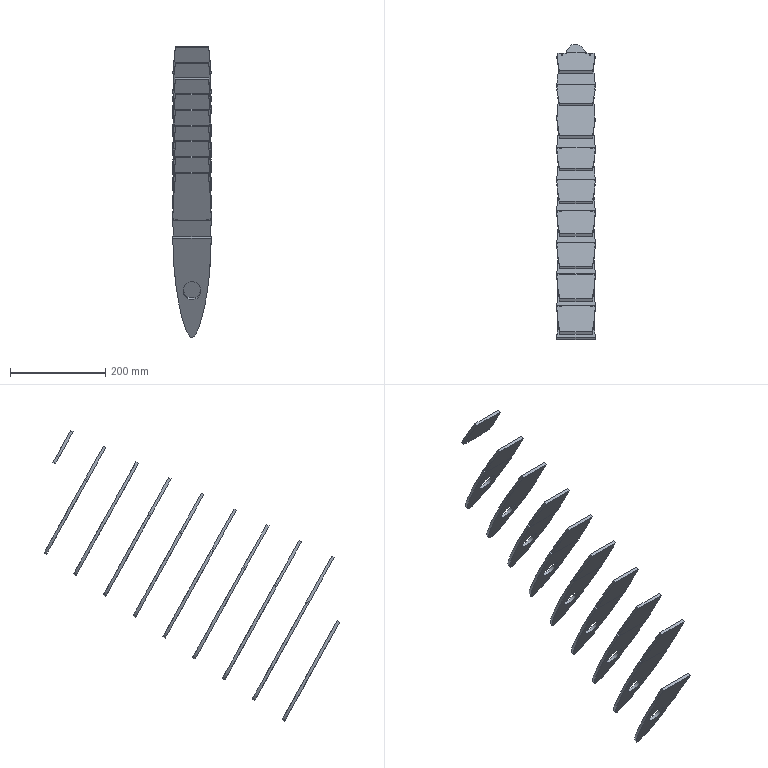Part | SolidWorks | features BaseBody 17 | 17 solids | 193 faces | box 80.78 x 620.956 x 611.862 mm | volume 997682 mm3 | plane 150 | spline 43